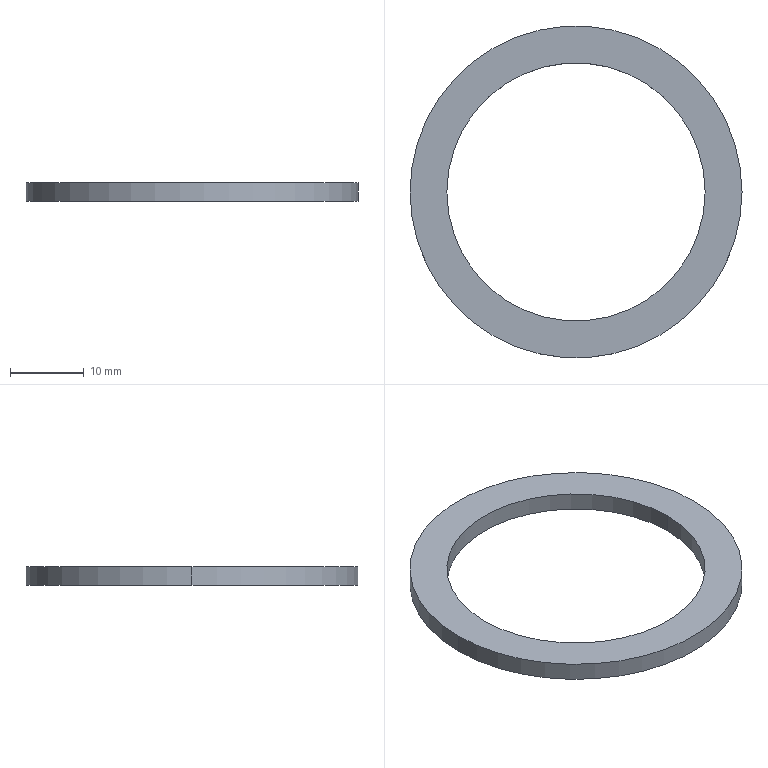Part | SolidWorks | features Extrusion 1 | 1 solid | 6 faces | box 45 x 45 x 2.5 mm | volume 1571 mm3 | cylinder 4 | plane 2 | commonest cylinder face diameters 35 x2 45 x2
STEP:
#1=CARTESIAN_POINT('',(-17.5,0.,2.5));
#2=VERTEX_POINT('',#1);
#3=CARTESIAN_POINT('',(17.5,0.,2.5));
#4=VERTEX_POINT('',#3);
#5=CARTESIAN_POINT('',(0.,0.,2.5));
#6=DIRECTION('',(0.,0.,1.));
#7=DIRECTION('',(1.,0.,0.));
#8=AXIS2_PLACEMENT_3D('',#5,#6,#7);
#9=CIRCLE('',#8,17.5);
#10=EDGE_CURVE('',#2,#4,#9,.T.);
#11=ORIENTED_EDGE('',*,*,#10,.T.);
#12=CARTESIAN_POINT('',(17.5,0.,0.));
#13=VERTEX_POINT('',#12);
#14=CARTESIAN_POINT('',(17.5,0.,2.5));
#15=DIRECTION('',(0.,0.,-1.));
#16=VECTOR('',#15,1000.);
#17=LINE('',#14,#16);
#18=EDGE_CURVE('',#4,#13,#17,.T.);
#19=ORIENTED_EDGE('',*,*,#18,.T.);
#20=CARTESIAN_POINT('',(-17.5,0.,0.));
#21=VERTEX_POINT('',#20);
#22=CARTESIAN_POINT('',(0.,0.,0.));
#23=DIRECTION('',(0.,0.,1.));
#24=DIRECTION('',(1.,0.,0.));
#25=AXIS2_PLACEMENT_3D('',#22,#23,#24);
#26=CIRCLE('',#25,17.5);
#27=EDGE_CURVE('',#21,#13,#26,.T.);
#28=ORIENTED_EDGE('',*,*,#27,.F.);
#29=CARTESIAN_POINT('',(-17.5,0.,2.5));
#30=DIRECTION('',(0.,0.,-1.));
#31=VECTOR('',#30,1000.);
#32=LINE('',#29,#31);
#33=EDGE_CURVE('',#2,#21,#32,.T.);
#34=ORIENTED_EDGE('',*,*,#33,.F.);
#35=EDGE_LOOP('',(#11,#19,#28,#34));
#36=FACE_OUTER_BOUND('',#35,.T.);
#37=CARTESIAN_POINT('',(0.,0.,2.5));
#38=DIRECTION('',(0.,0.,-1.));
#39=DIRECTION('',(-1.,0.,0.));
#40=AXIS2_PLACEMENT_3D('',#37,#38,#39);
#41=CYLINDRICAL_SURFACE('',#40,17.5);
#42=ADVANCED_FACE('',(#36),#41,.F.);
#43=CARTESIAN_POINT('',(22.5,0.,2.5));
#44=VERTEX_POINT('',#43);
#45=CARTESIAN_POINT('',(-22.5,0.,2.5));
#46=VERTEX_POINT('',#45);
#47=CARTESIAN_POINT('',(0.,0.,2.5));
#48=DIRECTION('',(0.,0.,1.));
#49=DIRECTION('',(1.,0.,0.));
#50=AXIS2_PLACEMENT_3D('',#47,#48,#49);
#51=CIRCLE('',#50,22.5);
#52=EDGE_CURVE('',#44,#46,#51,.T.);
#53=ORIENTED_EDGE('',*,*,#52,.F.);
#54=CARTESIAN_POINT('',(22.5,0.,0.));
#55=VERTEX_POINT('',#54);
#56=CARTESIAN_POINT('',(22.5,0.,2.5));
#57=DIRECTION('',(0.,0.,-1.));
#58=VECTOR('',#57,1000.);
#59=LINE('',#56,#58);
#60=EDGE_CURVE('',#44,#55,#59,.T.);
#61=ORIENTED_EDGE('',*,*,#60,.T.);
#62=CARTESIAN_POINT('',(-22.5,0.,0.));
#63=VERTEX_POINT('',#62);
#64=CARTESIAN_POINT('',(0.,0.,0.));
#65=DIRECTION('',(0.,0.,1.));
#66=DIRECTION('',(1.,0.,0.));
#67=AXIS2_PLACEMENT_3D('',#64,#65,#66);
#68=CIRCLE('',#67,22.5);
#69=EDGE_CURVE('',#55,#63,#68,.T.);
#70=ORIENTED_EDGE('',*,*,#69,.T.);
#71=CARTESIAN_POINT('',(-22.5,0.,2.5));
#72=DIRECTION('',(0.,0.,-1.));
#73=VECTOR('',#72,1000.);
#74=LINE('',#71,#73);
#75=EDGE_CURVE('',#46,#63,#74,.T.);
#76=ORIENTED_EDGE('',*,*,#75,.F.);
#77=EDGE_LOOP('',(#53,#61,#70,#76));
#78=FACE_OUTER_BOUND('',#77,.T.);
#79=CARTESIAN_POINT('',(0.,0.,2.5));
#80=DIRECTION('',(0.,0.,-1.));
#81=DIRECTION('',(-1.,0.,0.));
#82=AXIS2_PLACEMENT_3D('',#79,#80,#81);
#83=CYLINDRICAL_SURFACE('',#82,22.5);
#84=ADVANCED_FACE('',(#78),#83,.T.);
#85=CARTESIAN_POINT('',(0.,0.,2.5));
#86=DIRECTION('',(0.,0.,1.));
#87=DIRECTION('',(1.,0.,0.));
#88=AXIS2_PLACEMENT_3D('',#85,#86,#87);
#89=CIRCLE('',#88,22.5);
#90=EDGE_CURVE('',#46,#44,#89,.T.);
#91=ORIENTED_EDGE('',*,*,#90,.T.);
#92=ORIENTED_EDGE('',*,*,#52,.T.);
#93=EDGE_LOOP('',(#91,#92));
#94=FACE_OUTER_BOUND('',#93,.T.);
#95=ORIENTED_EDGE('',*,*,#10,.F.);
#96=CARTESIAN_POINT('',(0.,0.,2.5));
#97=DIRECTION('',(0.,0.,1.));
#98=DIRECTION('',(1.,0.,0.));
#99=AXIS2_PLACEMENT_3D('',#96,#97,#98);
#100=CIRCLE('',#99,17.5);
#101=EDGE_CURVE('',#4,#2,#100,.T.);
#102=ORIENTED_EDGE('',*,*,#101,.F.);
#103=EDGE_LOOP('',(#95,#102));
#104=FACE_BOUND('',#103,.T.);
#105=CARTESIAN_POINT('',(0.,0.,2.5));
#106=DIRECTION('',(0.,0.,1.));
#107=DIRECTION('',(1.,0.,0.));
#108=AXIS2_PLACEMENT_3D('',#105,#106,#107);
#109=PLANE('',#108);
#110=ADVANCED_FACE('',(#94,#104),#109,.T.);
#111=CARTESIAN_POINT('',(0.,0.,0.));
#112=DIRECTION('',(0.,0.,1.));
#113=DIRECTION('',(1.,0.,0.));
#114=AXIS2_PLACEMENT_3D('',#111,#112,#113);
#115=CIRCLE('',#114,22.5);
#116=EDGE_CURVE('',#63,#55,#115,.T.);
#117=ORIENTED_EDGE('',*,*,#116,.F.);
#118=ORIENTED_EDGE('',*,*,#69,.F.);
#119=EDGE_LOOP('',(#117,#118));
#120=FACE_OUTER_BOUND('',#119,.T.);
#121=ORIENTED_EDGE('',*,*,#27,.T.);
#122=CARTESIAN_POINT('',(0.,0.,0.));
#123=DIRECTION('',(0.,0.,1.));
#124=DIRECTION('',(1.,0.,0.));
#125=AXIS2_PLACEMENT_3D('',#122,#123,#124);
#126=CIRCLE('',#125,17.5);
#127=EDGE_CURVE('',#13,#21,#126,.T.);
#128=ORIENTED_EDGE('',*,*,#127,.T.);
#129=EDGE_LOOP('',(#121,#128));
#130=FACE_BOUND('',#129,.T.);
#131=CARTESIAN_POINT('',(0.,0.,0.));
#132=DIRECTION('',(0.,0.,1.));
#133=DIRECTION('',(1.,0.,0.));
#134=AXIS2_PLACEMENT_3D('',#131,#132,#133);
#135=PLANE('',#134);
#136=ADVANCED_FACE('',(#120,#130),#135,.F.);
#137=ORIENTED_EDGE('',*,*,#60,.F.);
#138=ORIENTED_EDGE('',*,*,#90,.F.);
#139=ORIENTED_EDGE('',*,*,#75,.T.);
#140=ORIENTED_EDGE('',*,*,#116,.T.);
#141=EDGE_LOOP('',(#137,#138,#139,#140));
#142=FACE_OUTER_BOUND('',#141,.T.);
#143=CARTESIAN_POINT('',(0.,0.,2.5));
#144=DIRECTION('',(0.,0.,-1.));
#145=DIRECTION('',(-1.,0.,0.));
#146=AXIS2_PLACEMENT_3D('',#143,#144,#145);
#147=CYLINDRICAL_SURFACE('',#146,22.5);
#148=ADVANCED_FACE('',(#142),#147,.T.);
#149=ORIENTED_EDGE('',*,*,#18,.F.);
#150=ORIENTED_EDGE('',*,*,#101,.T.);
#151=ORIENTED_EDGE('',*,*,#33,.T.);
#152=ORIENTED_EDGE('',*,*,#127,.F.);
#153=EDGE_LOOP('',(#149,#150,#151,#152));
#154=FACE_OUTER_BOUND('',#153,.T.);
#155=CARTESIAN_POINT('',(0.,0.,2.5));
#156=DIRECTION('',(0.,0.,-1.));
#157=DIRECTION('',(-1.,0.,0.));
#158=AXIS2_PLACEMENT_3D('',#155,#156,#157);
#159=CYLINDRICAL_SURFACE('',#158,17.5);
#160=ADVANCED_FACE('',(#154),#159,.F.);
#161=CLOSED_SHELL('',(#42,#84,#110,#136,#148,#160));
#162=MANIFOLD_SOLID_BREP('',#161);
#163=CARTESIAN_POINT('',(0.,0.,0.));
#164=DIRECTION('',(0.,0.,1.));
#165=DIRECTION('',(1.,0.,0.));
#166=AXIS2_PLACEMENT_3D('',#163,#164,#165);
#167=(LENGTH_UNIT()NAMED_UNIT(*)SI_UNIT(.MILLI.,.METRE.));
#168=UNCERTAINTY_MEASURE_WITH_UNIT(LENGTH_MEASURE(0.00001),#167,'','');
#169=(NAMED_UNIT(*)PLANE_ANGLE_UNIT()SI_UNIT($,.RADIAN.));
#170=(NAMED_UNIT(*)SI_UNIT($,.STERADIAN.)SOLID_ANGLE_UNIT());
#171=(GEOMETRIC_REPRESENTATION_CONTEXT(3)GLOBAL_UNCERTAINTY_ASSIGNED_CONTEXT((#168))GLOBAL_UNIT_ASSIGNED_CONTEXT((#167,#169,#170))REPRESENTATION_CONTEXT('',''));
#172=ADVANCED_BREP_SHAPE_REPRESENTATION('',(#162,#166),#171);